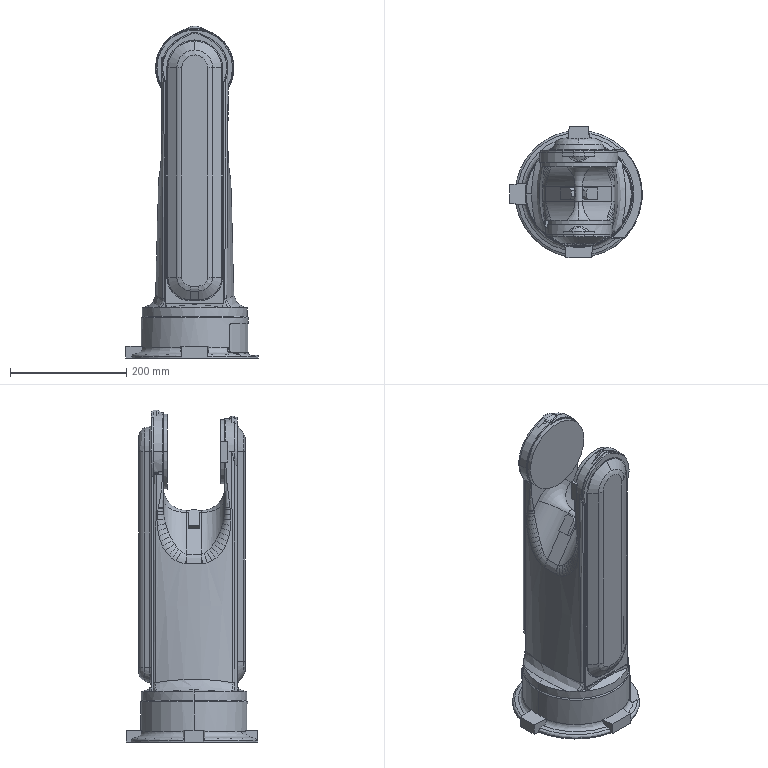Part | STEP file | Link4 | 1 solid | 304 faces | box 228 x 227 x 571.1 mm | volume 9720047 mm3 | spline 125 | plane 82 | cylinder 57 | cone 20 | torus 18 | sphere 2 | commonest cylinder face diameters 6 x10 30 x6 110 x5 4 x4 10 x4 80 x4